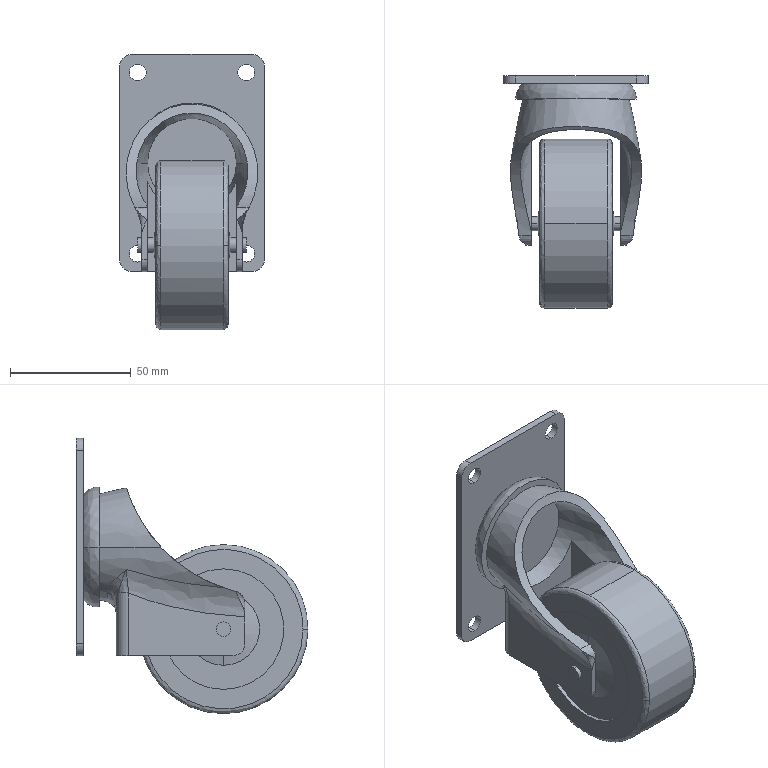Part | STEP file | Foot caster | 2 solids | 88 faces | box 60 x 96 x 114 mm | volume 163326 mm3 | cylinder 31 | plane 26 | spline 25 | cone 6 | commonest cylinder face diameters 6 x8 7 x8 10 x8 50 x4 70 x2 127.86 x1